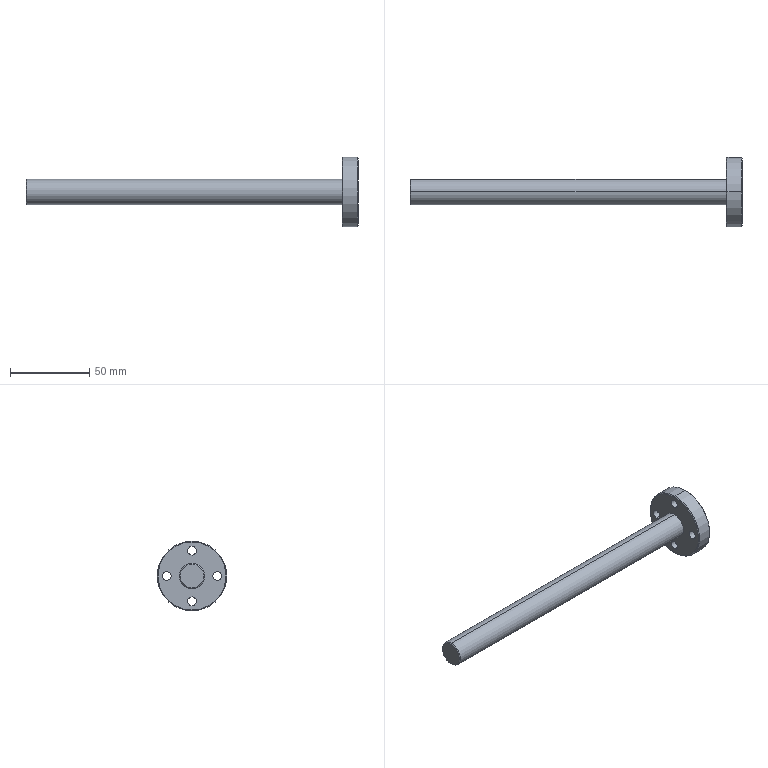Part | STEP file | shaft 9_SUS304 | 1 solid | 21 faces | box 210 x 44 x 44 mm | volume 54427 mm3 | cylinder 12 | cone 6 | plane 3 | commonest cylinder face diameters 5.5 x8 16 x2 44 x2